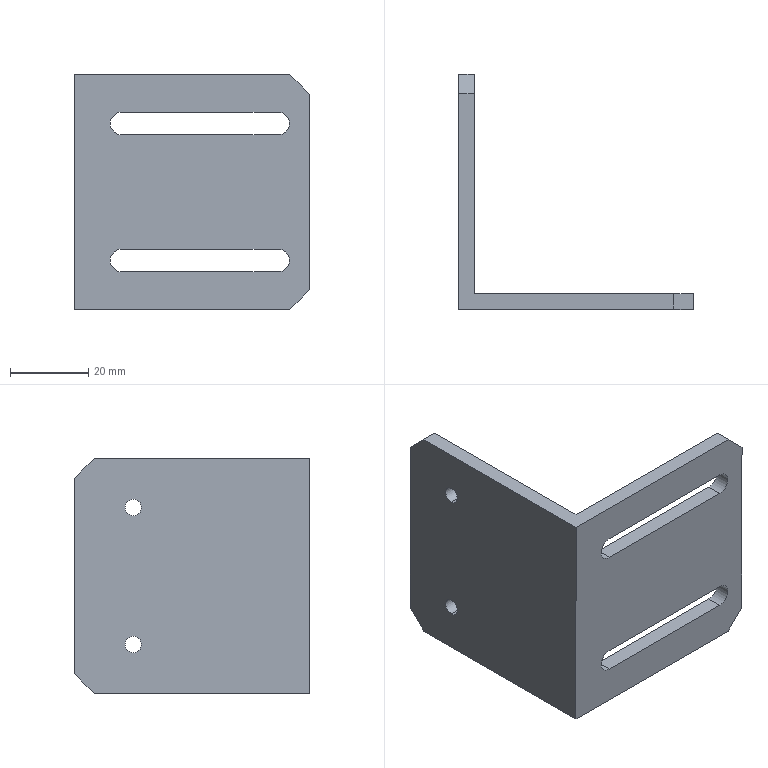Part | SolidWorks | features HoleWzd 2, Chamfer 1, Extrusion 1 | 1 solid | 24 faces | box 60 x 60 x 60 mm | volume 25462 mm3 | plane 16 | cylinder 8 | commonest cylinder face diameters 4.2 x4 5.8 x4
STEP:
#1=CARTESIAN_POINT('',(0.,45.,19.6));
#2=VERTEX_POINT('',#1);
#3=CARTESIAN_POINT('',(0.,45.,15.4));
#4=VERTEX_POINT('',#3);
#5=CARTESIAN_POINT('',(0.,45.,17.5));
#6=DIRECTION('',(1.,0.,0.));
#7=DIRECTION('',(0.,0.,-1.));
#8=AXIS2_PLACEMENT_3D('',#5,#6,#7);
#9=CIRCLE('',#8,2.1);
#10=EDGE_CURVE('',#2,#4,#9,.T.);
#11=ORIENTED_EDGE('',*,*,#10,.F.);
#12=CARTESIAN_POINT('',(4.,45.,19.6));
#13=VERTEX_POINT('',#12);
#14=CARTESIAN_POINT('',(4.,45.,19.6));
#15=DIRECTION('',(1.,0.,0.));
#16=VECTOR('',#15,1000.);
#17=LINE('',#14,#16);
#18=EDGE_CURVE('',#2,#13,#17,.T.);
#19=ORIENTED_EDGE('',*,*,#18,.T.);
#20=CARTESIAN_POINT('',(4.,45.,15.4));
#21=VERTEX_POINT('',#20);
#22=CARTESIAN_POINT('',(4.,45.,17.5));
#23=DIRECTION('',(1.,0.,0.));
#24=DIRECTION('',(0.,0.,-1.));
#25=AXIS2_PLACEMENT_3D('',#22,#23,#24);
#26=CIRCLE('',#25,2.1);
#27=EDGE_CURVE('',#13,#21,#26,.T.);
#28=ORIENTED_EDGE('',*,*,#27,.T.);
#29=CARTESIAN_POINT('',(4.,45.,15.4));
#30=DIRECTION('',(1.,0.,0.));
#31=VECTOR('',#30,1000.);
#32=LINE('',#29,#31);
#33=EDGE_CURVE('',#4,#21,#32,.T.);
#34=ORIENTED_EDGE('',*,*,#33,.F.);
#35=EDGE_LOOP('',(#11,#19,#28,#34));
#36=FACE_OUTER_BOUND('',#35,.T.);
#37=CARTESIAN_POINT('',(4.,45.,17.5));
#38=DIRECTION('',(1.,0.,0.));
#39=DIRECTION('',(0.,0.,-1.));
#40=AXIS2_PLACEMENT_3D('',#37,#38,#39);
#41=CYLINDRICAL_SURFACE('',#40,2.1);
#42=ADVANCED_FACE('',(#36),#41,.F.);
#43=CARTESIAN_POINT('',(0.,45.,-15.4));
#44=VERTEX_POINT('',#43);
#45=CARTESIAN_POINT('',(0.,45.,-19.6));
#46=VERTEX_POINT('',#45);
#47=CARTESIAN_POINT('',(0.,45.,-17.5));
#48=DIRECTION('',(1.,0.,0.));
#49=DIRECTION('',(0.,0.,-1.));
#50=AXIS2_PLACEMENT_3D('',#47,#48,#49);
#51=CIRCLE('',#50,2.1);
#52=EDGE_CURVE('',#44,#46,#51,.T.);
#53=ORIENTED_EDGE('',*,*,#52,.F.);
#54=CARTESIAN_POINT('',(4.,45.,-15.4));
#55=VERTEX_POINT('',#54);
#56=CARTESIAN_POINT('',(4.,45.,-15.4));
#57=DIRECTION('',(1.,0.,0.));
#58=VECTOR('',#57,1000.);
#59=LINE('',#56,#58);
#60=EDGE_CURVE('',#44,#55,#59,.T.);
#61=ORIENTED_EDGE('',*,*,#60,.T.);
#62=CARTESIAN_POINT('',(4.,45.,-19.6));
#63=VERTEX_POINT('',#62);
#64=CARTESIAN_POINT('',(4.,45.,-17.5));
#65=DIRECTION('',(1.,0.,0.));
#66=DIRECTION('',(0.,0.,-1.));
#67=AXIS2_PLACEMENT_3D('',#64,#65,#66);
#68=CIRCLE('',#67,2.1);
#69=EDGE_CURVE('',#55,#63,#68,.T.);
#70=ORIENTED_EDGE('',*,*,#69,.T.);
#71=CARTESIAN_POINT('',(4.,45.,-19.6));
#72=DIRECTION('',(1.,0.,0.));
#73=VECTOR('',#72,1000.);
#74=LINE('',#71,#73);
#75=EDGE_CURVE('',#46,#63,#74,.T.);
#76=ORIENTED_EDGE('',*,*,#75,.F.);
#77=EDGE_LOOP('',(#53,#61,#70,#76));
#78=FACE_OUTER_BOUND('',#77,.T.);
#79=CARTESIAN_POINT('',(4.,45.,-17.5));
#80=DIRECTION('',(1.,0.,0.));
#81=DIRECTION('',(0.,0.,-1.));
#82=AXIS2_PLACEMENT_3D('',#79,#80,#81);
#83=CYLINDRICAL_SURFACE('',#82,2.1);
#84=ADVANCED_FACE('',(#78),#83,.F.);
#85=CARTESIAN_POINT('',(12.,0.,-20.4));
#86=VERTEX_POINT('',#85);
#87=CARTESIAN_POINT('',(52.,0.,-20.4));
#88=VERTEX_POINT('',#87);
#89=CARTESIAN_POINT('',(12.,0.,-20.4));
#90=DIRECTION('',(1.,0.,0.));
#91=VECTOR('',#90,1000.);
#92=LINE('',#89,#91);
#93=EDGE_CURVE('',#86,#88,#92,.T.);
#94=ORIENTED_EDGE('',*,*,#93,.F.);
#95=CARTESIAN_POINT('',(12.,0.,-14.6));
#96=VERTEX_POINT('',#95);
#97=CARTESIAN_POINT('',(12.,0.,-17.5));
#98=DIRECTION('',(0.,1.,0.));
#99=DIRECTION('',(0.,0.,1.));
#100=AXIS2_PLACEMENT_3D('',#97,#98,#99);
#101=CIRCLE('',#100,2.9);
#102=EDGE_CURVE('',#86,#96,#101,.T.);
#103=ORIENTED_EDGE('',*,*,#102,.T.);
#104=CARTESIAN_POINT('',(52.,0.,-14.6));
#105=VERTEX_POINT('',#104);
#106=CARTESIAN_POINT('',(12.,0.,-14.6));
#107=DIRECTION('',(1.,0.,0.));
#108=VECTOR('',#107,1000.);
#109=LINE('',#106,#108);
#110=EDGE_CURVE('',#96,#105,#109,.T.);
#111=ORIENTED_EDGE('',*,*,#110,.T.);
#112=CARTESIAN_POINT('',(52.,0.,-17.5));
#113=DIRECTION('',(0.,1.,0.));
#114=DIRECTION('',(0.,0.,1.));
#115=AXIS2_PLACEMENT_3D('',#112,#113,#114);
#116=CIRCLE('',#115,2.9);
#117=EDGE_CURVE('',#105,#88,#116,.T.);
#118=ORIENTED_EDGE('',*,*,#117,.T.);
#119=EDGE_LOOP('',(#94,#103,#111,#118));
#120=FACE_BOUND('',#119,.T.);
#121=CARTESIAN_POINT('',(12.,0.,14.6));
#122=VERTEX_POINT('',#121);
#123=CARTESIAN_POINT('',(12.,0.,20.4));
#124=VERTEX_POINT('',#123);
#125=CARTESIAN_POINT('',(12.,0.,17.5));
#126=DIRECTION('',(0.,1.,0.));
#127=DIRECTION('',(0.,0.,1.));
#128=AXIS2_PLACEMENT_3D('',#125,#126,#127);
#129=CIRCLE('',#128,2.9);
#130=EDGE_CURVE('',#122,#124,#129,.T.);
#131=ORIENTED_EDGE('',*,*,#130,.T.);
#132=CARTESIAN_POINT('',(52.,0.,20.4));
#133=VERTEX_POINT('',#132);
#134=CARTESIAN_POINT('',(12.,0.,20.4));
#135=DIRECTION('',(1.,0.,0.));
#136=VECTOR('',#135,1000.);
#137=LINE('',#134,#136);
#138=EDGE_CURVE('',#124,#133,#137,.T.);
#139=ORIENTED_EDGE('',*,*,#138,.T.);
#140=CARTESIAN_POINT('',(52.,0.,14.6));
#141=VERTEX_POINT('',#140);
#142=CARTESIAN_POINT('',(52.,0.,17.5));
#143=DIRECTION('',(0.,1.,0.));
#144=DIRECTION('',(0.,0.,1.));
#145=AXIS2_PLACEMENT_3D('',#142,#143,#144);
#146=CIRCLE('',#145,2.9);
#147=EDGE_CURVE('',#133,#141,#146,.T.);
#148=ORIENTED_EDGE('',*,*,#147,.T.);
#149=CARTESIAN_POINT('',(12.,0.,14.6));
#150=DIRECTION('',(1.,0.,0.));
#151=VECTOR('',#150,1000.);
#152=LINE('',#149,#151);
#153=EDGE_CURVE('',#122,#141,#152,.T.);
#154=ORIENTED_EDGE('',*,*,#153,.F.);
#155=EDGE_LOOP('',(#131,#139,#148,#154));
#156=FACE_BOUND('',#155,.T.);
#157=CARTESIAN_POINT('',(60.,0.,25.));
#158=VERTEX_POINT('',#157);
#159=CARTESIAN_POINT('',(60.,0.,-25.));
#160=VERTEX_POINT('',#159);
#161=CARTESIAN_POINT('',(60.,0.,30.));
#162=DIRECTION('',(0.,0.,-1.));
#163=VECTOR('',#162,1000.);
#164=LINE('',#161,#163);
#165=EDGE_CURVE('',#158,#160,#164,.T.);
#166=ORIENTED_EDGE('',*,*,#165,.F.);
#167=CARTESIAN_POINT('',(55.,0.,30.));
#168=VERTEX_POINT('',#167);
#169=CARTESIAN_POINT('',(55.,0.,30.));
#170=DIRECTION('',(-0.7071,0.,0.7071));
#171=VECTOR('',#170,1000.);
#172=LINE('',#169,#171);
#173=EDGE_CURVE('',#158,#168,#172,.T.);
#174=ORIENTED_EDGE('',*,*,#173,.T.);
#175=CARTESIAN_POINT('',(0.,0.,30.));
#176=VERTEX_POINT('',#175);
#177=CARTESIAN_POINT('',(60.,0.,30.));
#178=DIRECTION('',(1.,0.,0.));
#179=VECTOR('',#178,1000.);
#180=LINE('',#177,#179);
#181=EDGE_CURVE('',#176,#168,#180,.T.);
#182=ORIENTED_EDGE('',*,*,#181,.F.);
#183=CARTESIAN_POINT('',(0.,0.,-30.));
#184=VERTEX_POINT('',#183);
#185=CARTESIAN_POINT('',(0.,0.,30.));
#186=DIRECTION('',(0.,0.,-1.));
#187=VECTOR('',#186,1000.);
#188=LINE('',#185,#187);
#189=EDGE_CURVE('',#176,#184,#188,.T.);
#190=ORIENTED_EDGE('',*,*,#189,.T.);
#191=CARTESIAN_POINT('',(55.,0.,-30.));
#192=VERTEX_POINT('',#191);
#193=CARTESIAN_POINT('',(60.,0.,-30.));
#194=DIRECTION('',(1.,0.,0.));
#195=VECTOR('',#194,1000.);
#196=LINE('',#193,#195);
#197=EDGE_CURVE('',#184,#192,#196,.T.);
#198=ORIENTED_EDGE('',*,*,#197,.T.);
#199=CARTESIAN_POINT('',(60.,0.,-25.));
#200=DIRECTION('',(0.7071,0.,0.7071));
#201=VECTOR('',#200,1000.);
#202=LINE('',#199,#201);
#203=EDGE_CURVE('',#192,#160,#202,.T.);
#204=ORIENTED_EDGE('',*,*,#203,.T.);
#205=EDGE_LOOP('',(#166,#174,#182,#190,#198,#204));
#206=FACE_OUTER_BOUND('',#205,.T.);
#207=CARTESIAN_POINT('',(60.,0.,30.));
#208=DIRECTION('',(0.,1.,0.));
#209=DIRECTION('',(-1.,0.,0.));
#210=AXIS2_PLACEMENT_3D('',#207,#208,#209);
#211=PLANE('',#210);
#212=ADVANCED_FACE('',(#120,#156,#206),#211,.F.);
#213=CARTESIAN_POINT('',(60.,4.,25.));
#214=VERTEX_POINT('',#213);
#215=CARTESIAN_POINT('',(60.,4.,-25.));
#216=VERTEX_POINT('',#215);
#217=CARTESIAN_POINT('',(60.,4.,30.));
#218=DIRECTION('',(0.,0.,-1.));
#219=VECTOR('',#218,1000.);
#220=LINE('',#217,#219);
#221=EDGE_CURVE('',#214,#216,#220,.T.);
#222=ORIENTED_EDGE('',*,*,#221,.F.);
#223=CARTESIAN_POINT('',(60.,4.,25.));
#224=DIRECTION('',(0.,-1.,0.));
#225=VECTOR('',#224,1000.);
#226=LINE('',#223,#225);
#227=EDGE_CURVE('',#214,#158,#226,.T.);
#228=ORIENTED_EDGE('',*,*,#227,.T.);
#229=ORIENTED_EDGE('',*,*,#165,.T.);
#230=CARTESIAN_POINT('',(60.,4.,-25.));
#231=DIRECTION('',(0.,1.,0.));
#232=VECTOR('',#231,1000.);
#233=LINE('',#230,#232);
#234=EDGE_CURVE('',#160,#216,#233,.T.);
#235=ORIENTED_EDGE('',*,*,#234,.T.);
#236=EDGE_LOOP('',(#222,#228,#229,#235));
#237=FACE_OUTER_BOUND('',#236,.T.);
#238=CARTESIAN_POINT('',(60.,4.,30.));
#239=DIRECTION('',(-1.,0.,0.));
#240=DIRECTION('',(0.,0.,1.));
#241=AXIS2_PLACEMENT_3D('',#238,#239,#240);
#242=PLANE('',#241);
#243=ADVANCED_FACE('',(#237),#242,.F.);
#244=CARTESIAN_POINT('',(12.,4.,-20.4));
#245=VERTEX_POINT('',#244);
#246=CARTESIAN_POINT('',(12.,4.,-14.6));
#247=VERTEX_POINT('',#246);
#248=CARTESIAN_POINT('',(12.,4.,-17.5));
#249=DIRECTION('',(0.,1.,0.));
#250=DIRECTION('',(0.,0.,1.));
#251=AXIS2_PLACEMENT_3D('',#248,#249,#250);
#252=CIRCLE('',#251,2.9);
#253=EDGE_CURVE('',#245,#247,#252,.T.);
#254=ORIENTED_EDGE('',*,*,#253,.F.);
#255=CARTESIAN_POINT('',(52.,4.,-20.4));
#256=VERTEX_POINT('',#255);
#257=CARTESIAN_POINT('',(12.,4.,-20.4));
#258=DIRECTION('',(1.,0.,0.));
#259=VECTOR('',#258,1000.);
#260=LINE('',#257,#259);
#261=EDGE_CURVE('',#245,#256,#260,.T.);
#262=ORIENTED_EDGE('',*,*,#261,.T.);
#263=CARTESIAN_POINT('',(52.,4.,-14.6));
#264=VERTEX_POINT('',#263);
#265=CARTESIAN_POINT('',(52.,4.,-17.5));
#266=DIRECTION('',(0.,1.,0.));
#267=DIRECTION('',(0.,0.,1.));
#268=AXIS2_PLACEMENT_3D('',#265,#266,#267);
#269=CIRCLE('',#268,2.9);
#270=EDGE_CURVE('',#264,#256,#269,.T.);
#271=ORIENTED_EDGE('',*,*,#270,.F.);
#272=CARTESIAN_POINT('',(12.,4.,-14.6));
#273=DIRECTION('',(1.,0.,0.));
#274=VECTOR('',#273,1000.);
#275=LINE('',#272,#274);
#276=EDGE_CURVE('',#247,#264,#275,.T.);
#277=ORIENTED_EDGE('',*,*,#276,.F.);
#278=EDGE_LOOP('',(#254,#262,#271,#277));
#279=FACE_BOUND('',#278,.T.);
#280=CARTESIAN_POINT('',(12.,4.,14.6));
#281=VERTEX_POINT('',#280);
#282=CARTESIAN_POINT('',(52.,4.,14.6));
#283=VERTEX_POINT('',#282);
#284=CARTESIAN_POINT('',(12.,4.,14.6));
#285=DIRECTION('',(1.,0.,0.));
#286=VECTOR('',#285,1000.);
#287=LINE('',#284,#286);
#288=EDGE_CURVE('',#281,#283,#287,.T.);
#289=ORIENTED_EDGE('',*,*,#288,.T.);
#290=CARTESIAN_POINT('',(52.,4.,20.4));
#291=VERTEX_POINT('',#290);
#292=CARTESIAN_POINT('',(52.,4.,17.5));
#293=DIRECTION('',(0.,1.,0.));
#294=DIRECTION('',(0.,0.,1.));
#295=AXIS2_PLACEMENT_3D('',#292,#293,#294);
#296=CIRCLE('',#295,2.9);
#297=EDGE_CURVE('',#291,#283,#296,.T.);
#298=ORIENTED_EDGE('',*,*,#297,.F.);
#299=CARTESIAN_POINT('',(12.,4.,20.4));
#300=VERTEX_POINT('',#299);
#301=CARTESIAN_POINT('',(12.,4.,20.4));
#302=DIRECTION('',(1.,0.,0.));
#303=VECTOR('',#302,1000.);
#304=LINE('',#301,#303);
#305=EDGE_CURVE('',#300,#291,#304,.T.);
#306=ORIENTED_EDGE('',*,*,#305,.F.);
#307=CARTESIAN_POINT('',(12.,4.,17.5));
#308=DIRECTION('',(0.,1.,0.));
#309=DIRECTION('',(0.,0.,1.));
#310=AXIS2_PLACEMENT_3D('',#307,#308,#309);
#311=CIRCLE('',#310,2.9);
#312=EDGE_CURVE('',#281,#300,#311,.T.);
#313=ORIENTED_EDGE('',*,*,#312,.F.);
#314=EDGE_LOOP('',(#289,#298,#306,#313));
#315=FACE_BOUND('',#314,.T.);
#316=CARTESIAN_POINT('',(55.,4.,30.));
#317=VERTEX_POINT('',#316);
#318=CARTESIAN_POINT('',(4.,4.,30.));
#319=VERTEX_POINT('',#318);
#320=CARTESIAN_POINT('',(4.,4.,30.));
#321=DIRECTION('',(-1.,0.,0.));
#322=VECTOR('',#321,1000.);
#323=LINE('',#320,#322);
#324=EDGE_CURVE('',#317,#319,#323,.T.);
#325=ORIENTED_EDGE('',*,*,#324,.F.);
#326=CARTESIAN_POINT('',(55.,4.,30.));
#327=DIRECTION('',(0.7071,0.,-0.7071));
#328=VECTOR('',#327,1000.);
#329=LINE('',#326,#328);
#330=EDGE_CURVE('',#317,#214,#329,.T.);
#331=ORIENTED_EDGE('',*,*,#330,.T.);
#332=ORIENTED_EDGE('',*,*,#221,.T.);
#333=CARTESIAN_POINT('',(55.,4.,-30.));
#334=VERTEX_POINT('',#333);
#335=CARTESIAN_POINT('',(60.,4.,-25.));
#336=DIRECTION('',(-0.7071,0.,-0.7071));
#337=VECTOR('',#336,1000.);
#338=LINE('',#335,#337);
#339=EDGE_CURVE('',#216,#334,#338,.T.);
#340=ORIENTED_EDGE('',*,*,#339,.T.);
#341=CARTESIAN_POINT('',(4.,4.,-30.));
#342=VERTEX_POINT('',#341);
#343=CARTESIAN_POINT('',(4.,4.,-30.));
#344=DIRECTION('',(-1.,0.,0.));
#345=VECTOR('',#344,1000.);
#346=LINE('',#343,#345);
#347=EDGE_CURVE('',#334,#342,#346,.T.);
#348=ORIENTED_EDGE('',*,*,#347,.T.);
#349=CARTESIAN_POINT('',(4.,4.,30.));
#350=DIRECTION('',(0.,0.,-1.));
#351=VECTOR('',#350,1000.);
#352=LINE('',#349,#351);
#353=EDGE_CURVE('',#319,#342,#352,.T.);
#354=ORIENTED_EDGE('',*,*,#353,.F.);
#355=EDGE_LOOP('',(#325,#331,#332,#340,#348,#354));
#356=FACE_OUTER_BOUND('',#355,.T.);
#357=CARTESIAN_POINT('',(4.,4.,30.));
#358=DIRECTION('',(0.,-1.,0.));
#359=DIRECTION('',(0.,0.,-1.));
#360=AXIS2_PLACEMENT_3D('',#357,#358,#359);
#361=PLANE('',#360);
#362=ADVANCED_FACE('',(#279,#315,#356),#361,.F.);
#363=CARTESIAN_POINT('',(4.,45.,17.5));
#364=DIRECTION('',(1.,0.,0.));
#365=DIRECTION('',(0.,0.,-1.));
#366=AXIS2_PLACEMENT_3D('',#363,#364,#365);
#367=CIRCLE('',#366,2.1);
#368=EDGE_CURVE('',#21,#13,#367,.T.);
#369=ORIENTED_EDGE('',*,*,#368,.F.);
#370=ORIENTED_EDGE('',*,*,#27,.F.);
#371=EDGE_LOOP('',(#369,#370));
#372=FACE_BOUND('',#371,.T.);
#373=CARTESIAN_POINT('',(4.,45.,-17.5));
#374=DIRECTION('',(1.,0.,0.));
#375=DIRECTION('',(0.,0.,-1.));
#376=AXIS2_PLACEMENT_3D('',#373,#374,#375);
#377=CIRCLE('',#376,2.1);
#378=EDGE_CURVE('',#63,#55,#377,.T.);
#379=ORIENTED_EDGE('',*,*,#378,.F.);
#380=ORIENTED_EDGE('',*,*,#69,.F.);
#381=EDGE_LOOP('',(#379,#380));
#382=FACE_BOUND('',#381,.T.);
#383=CARTESIAN_POINT('',(4.,55.,-30.));
#384=VERTEX_POINT('',#383);
#385=CARTESIAN_POINT('',(4.,60.,-30.));
#386=DIRECTION('',(0.,1.,0.));
#387=VECTOR('',#386,1000.);
#388=LINE('',#385,#387);
#389=EDGE_CURVE('',#342,#384,#388,.T.);
#390=ORIENTED_EDGE('',*,*,#389,.T.);
#391=CARTESIAN_POINT('',(4.,60.,-25.));
#392=VERTEX_POINT('',#391);
#393=CARTESIAN_POINT('',(4.,60.,-25.));
#394=DIRECTION('',(0.,0.7071,0.7071));
#395=VECTOR('',#394,1000.);
#396=LINE('',#393,#395);
#397=EDGE_CURVE('',#384,#392,#396,.T.);
#398=ORIENTED_EDGE('',*,*,#397,.T.);
#399=CARTESIAN_POINT('',(4.,60.,25.));
#400=VERTEX_POINT('',#399);
#401=CARTESIAN_POINT('',(4.,60.,30.));
#402=DIRECTION('',(0.,0.,-1.));
#403=VECTOR('',#402,1000.);
#404=LINE('',#401,#403);
#405=EDGE_CURVE('',#400,#392,#404,.T.);
#406=ORIENTED_EDGE('',*,*,#405,.F.);
#407=CARTESIAN_POINT('',(4.,55.,30.));
#408=VERTEX_POINT('',#407);
#409=CARTESIAN_POINT('',(4.,55.,30.));
#410=DIRECTION('',(0.,-0.7071,0.7071));
#411=VECTOR('',#410,1000.);
#412=LINE('',#409,#411);
#413=EDGE_CURVE('',#400,#408,#412,.T.);
#414=ORIENTED_EDGE('',*,*,#413,.T.);
#415=CARTESIAN_POINT('',(4.,60.,30.));
#416=DIRECTION('',(0.,1.,0.));
#417=VECTOR('',#416,1000.);
#418=LINE('',#415,#417);
#419=EDGE_CURVE('',#319,#408,#418,.T.);
#420=ORIENTED_EDGE('',*,*,#419,.F.);
#421=ORIENTED_EDGE('',*,*,#353,.T.);
#422=EDGE_LOOP('',(#390,#398,#406,#414,#420,#421));
#423=FACE_OUTER_BOUND('',#422,.T.);
#424=CARTESIAN_POINT('',(4.,60.,30.));
#425=DIRECTION('',(-1.,0.,0.));
#426=DIRECTION('',(0.,-1.,0.));
#427=AXIS2_PLACEMENT_3D('',#424,#425,#426);
#428=PLANE('',#427);
#429=ADVANCED_FACE('',(#372,#382,#423),#428,.F.);
#430=ORIENTED_EDGE('',*,*,#405,.T.);
#431=CARTESIAN_POINT('',(0.,60.,-25.));
#432=VERTEX_POINT('',#431);
#433=CARTESIAN_POINT('',(0.,60.,-25.));
#434=DIRECTION('',(-1.,0.,0.));
#435=VECTOR('',#434,1000.);
#436=LINE('',#433,#435);
#437=EDGE_CURVE('',#392,#432,#436,.T.);
#438=ORIENTED_EDGE('',*,*,#437,.T.);
#439=CARTESIAN_POINT('',(0.,60.,25.));
#440=VERTEX_POINT('',#439);
#441=CARTESIAN_POINT('',(0.,60.,30.));
#442=DIRECTION('',(0.,0.,-1.));
#443=VECTOR('',#442,1000.);
#444=LINE('',#441,#443);
#445=EDGE_CURVE('',#440,#432,#444,.T.);
#446=ORIENTED_EDGE('',*,*,#445,.F.);
#447=CARTESIAN_POINT('',(0.,60.,25.));
#448=DIRECTION('',(1.,0.,0.));
#449=VECTOR('',#448,1000.);
#450=LINE('',#447,#449);
#451=EDGE_CURVE('',#440,#400,#450,.T.);
#452=ORIENTED_EDGE('',*,*,#451,.T.);
#453=EDGE_LOOP('',(#430,#438,#446,#452));
#454=FACE_OUTER_BOUND('',#453,.T.);
#455=CARTESIAN_POINT('',(0.,60.,30.));
#456=DIRECTION('',(0.,-1.,0.));
#457=DIRECTION('',(0.,0.,-1.));
#458=AXIS2_PLACEMENT_3D('',#455,#456,#457);
#459=PLANE('',#458);
#460=ADVANCED_FACE('',(#454),#459,.F.);
#461=CARTESIAN_POINT('',(0.,45.,17.5));
#462=DIRECTION('',(1.,0.,0.));
#463=DIRECTION('',(0.,0.,-1.));
#464=AXIS2_PLACEMENT_3D('',#461,#462,#463);
#465=CIRCLE('',#464,2.1);
#466=EDGE_CURVE('',#4,#2,#465,.T.);
#467=ORIENTED_EDGE('',*,*,#466,.T.);
#468=ORIENTED_EDGE('',*,*,#10,.T.);
#469=EDGE_LOOP('',(#467,#468));
#470=FACE_BOUND('',#469,.T.);
#471=CARTESIAN_POINT('',(0.,45.,-17.5));
#472=DIRECTION('',(1.,0.,0.));
#473=DIRECTION('',(0.,0.,-1.));
#474=AXIS2_PLACEMENT_3D('',#471,#472,#473);
#475=CIRCLE('',#474,2.1);
#476=EDGE_CURVE('',#46,#44,#475,.T.);
#477=ORIENTED_EDGE('',*,*,#476,.T.);
#478=ORIENTED_EDGE('',*,*,#52,.T.);
#479=EDGE_LOOP('',(#477,#478));
#480=FACE_BOUND('',#479,.T.);
#481=ORIENTED_EDGE('',*,*,#445,.T.);
#482=CARTESIAN_POINT('',(0.,55.,-30.));
#483=VERTEX_POINT('',#482);
#484=CARTESIAN_POINT('',(0.,60.,-25.));
#485=DIRECTION('',(0.,-0.7071,-0.7071));
#486=VECTOR('',#485,1000.);
#487=LINE('',#484,#486);
#488=EDGE_CURVE('',#432,#483,#487,.T.);
#489=ORIENTED_EDGE('',*,*,#488,.T.);
#490=CARTESIAN_POINT('',(0.,0.,-30.));
#491=DIRECTION('',(0.,-1.,0.));
#492=VECTOR('',#491,1000.);
#493=LINE('',#490,#492);
#494=EDGE_CURVE('',#483,#184,#493,.T.);
#495=ORIENTED_EDGE('',*,*,#494,.T.);
#496=ORIENTED_EDGE('',*,*,#189,.F.);
#497=CARTESIAN_POINT('',(0.,55.,30.));
#498=VERTEX_POINT('',#497);
#499=CARTESIAN_POINT('',(0.,0.,30.));
#500=DIRECTION('',(0.,-1.,0.));
#501=VECTOR('',#500,1000.);
#502=LINE('',#499,#501);
#503=EDGE_CURVE('',#498,#176,#502,.T.);
#504=ORIENTED_EDGE('',*,*,#503,.F.);
#505=CARTESIAN_POINT('',(0.,55.,30.));
#506=DIRECTION('',(0.,0.7071,-0.7071));
#507=VECTOR('',#506,1000.);
#508=LINE('',#505,#507);
#509=EDGE_CURVE('',#498,#440,#508,.T.);
#510=ORIENTED_EDGE('',*,*,#509,.T.);
#511=EDGE_LOOP('',(#481,#489,#495,#496,#504,#510));
#512=FACE_OUTER_BOUND('',#511,.T.);
#513=CARTESIAN_POINT('',(0.,0.,30.));
#514=DIRECTION('',(1.,0.,0.));
#515=DIRECTION('',(0.,0.,-1.));
#516=AXIS2_PLACEMENT_3D('',#513,#514,#515);
#517=PLANE('',#516);
#518=ADVANCED_FACE('',(#470,#480,#512),#517,.F.);
#519=ORIENTED_EDGE('',*,*,#181,.T.);
#520=CARTESIAN_POINT('',(55.,0.,30.));
#521=DIRECTION('',(0.,1.,0.));
#522=VECTOR('',#521,1000.);
#523=LINE('',#520,#522);
#524=EDGE_CURVE('',#168,#317,#523,.T.);
#525=ORIENTED_EDGE('',*,*,#524,.T.);
#526=ORIENTED_EDGE('',*,*,#324,.T.);
#527=ORIENTED_EDGE('',*,*,#419,.T.);
#528=CARTESIAN_POINT('',(0.,55.,30.));
#529=DIRECTION('',(-1.,0.,0.));
#530=VECTOR('',#529,1000.);
#531=LINE('',#528,#530);
#532=EDGE_CURVE('',#408,#498,#531,.T.);
#533=ORIENTED_EDGE('',*,*,#532,.T.);
#534=ORIENTED_EDGE('',*,*,#503,.T.);
#535=EDGE_LOOP('',(#519,#525,#526,#527,#533,#534));
#536=FACE_OUTER_BOUND('',#535,.T.);
#537=CARTESIAN_POINT('',(0.,0.,30.));
#538=DIRECTION('',(0.,0.,-1.));
#539=DIRECTION('',(-1.,0.,0.));
#540=AXIS2_PLACEMENT_3D('',#537,#538,#539);
#541=PLANE('',#540);
#542=ADVANCED_FACE('',(#536),#541,.F.);
#543=ORIENTED_EDGE('',*,*,#347,.F.);
#544=CARTESIAN_POINT('',(55.,0.,-30.));
#545=DIRECTION('',(0.,-1.,0.));
#546=VECTOR('',#545,1000.);
#547=LINE('',#544,#546);
#548=EDGE_CURVE('',#334,#192,#547,.T.);
#549=ORIENTED_EDGE('',*,*,#548,.T.);
#550=ORIENTED_EDGE('',*,*,#197,.F.);
#551=ORIENTED_EDGE('',*,*,#494,.F.);
#552=CARTESIAN_POINT('',(4.,55.,-30.));
#553=DIRECTION('',(1.,0.,0.));
#554=VECTOR('',#553,1000.);
#555=LINE('',#552,#554);
#556=EDGE_CURVE('',#483,#384,#555,.T.);
#557=ORIENTED_EDGE('',*,*,#556,.T.);
#558=ORIENTED_EDGE('',*,*,#389,.F.);
#559=EDGE_LOOP('',(#543,#549,#550,#551,#557,#558));
#560=FACE_OUTER_BOUND('',#559,.T.);
#561=CARTESIAN_POINT('',(0.,0.,-30.));
#562=DIRECTION('',(0.,0.,-1.));
#563=DIRECTION('',(-1.,0.,0.));
#564=AXIS2_PLACEMENT_3D('',#561,#562,#563);
#565=PLANE('',#564);
#566=ADVANCED_FACE('',(#560),#565,.T.);
#567=ORIENTED_EDGE('',*,*,#60,.F.);
#568=ORIENTED_EDGE('',*,*,#476,.F.);
#569=ORIENTED_EDGE('',*,*,#75,.T.);
#570=ORIENTED_EDGE('',*,*,#378,.T.);
#571=EDGE_LOOP('',(#567,#568,#569,#570));
#572=FACE_OUTER_BOUND('',#571,.T.);
#573=CARTESIAN_POINT('',(4.,45.,-17.5));
#574=DIRECTION('',(1.,0.,0.));
#575=DIRECTION('',(0.,0.,-1.));
#576=AXIS2_PLACEMENT_3D('',#573,#574,#575);
#577=CYLINDRICAL_SURFACE('',#576,2.1);
#578=ADVANCED_FACE('',(#572),#577,.F.);
#579=ORIENTED_EDGE('',*,*,#18,.F.);
#580=ORIENTED_EDGE('',*,*,#466,.F.);
#581=ORIENTED_EDGE('',*,*,#33,.T.);
#582=ORIENTED_EDGE('',*,*,#368,.T.);
#583=EDGE_LOOP('',(#579,#580,#581,#582));
#584=FACE_OUTER_BOUND('',#583,.T.);
#585=CARTESIAN_POINT('',(4.,45.,17.5));
#586=DIRECTION('',(1.,0.,0.));
#587=DIRECTION('',(0.,0.,-1.));
#588=AXIS2_PLACEMENT_3D('',#585,#586,#587);
#589=CYLINDRICAL_SURFACE('',#588,2.1);
#590=ADVANCED_FACE('',(#584),#589,.F.);
#591=ORIENTED_EDGE('',*,*,#147,.F.);
#592=CARTESIAN_POINT('',(52.,4.,20.4));
#593=DIRECTION('',(0.,-1.,0.));
#594=VECTOR('',#593,1000.);
#595=LINE('',#592,#594);
#596=EDGE_CURVE('',#291,#133,#595,.T.);
#597=ORIENTED_EDGE('',*,*,#596,.F.);
#598=ORIENTED_EDGE('',*,*,#297,.T.);
#599=CARTESIAN_POINT('',(52.,4.,14.6));
#600=DIRECTION('',(0.,1.,0.));
#601=VECTOR('',#600,1000.);
#602=LINE('',#599,#601);
#603=EDGE_CURVE('',#141,#283,#602,.T.);
#604=ORIENTED_EDGE('',*,*,#603,.F.);
#605=EDGE_LOOP('',(#591,#597,#598,#604));
#606=FACE_OUTER_BOUND('',#605,.T.);
#607=CARTESIAN_POINT('',(52.,4.,17.5));
#608=DIRECTION('',(0.,1.,0.));
#609=DIRECTION('',(0.,0.,1.));
#610=AXIS2_PLACEMENT_3D('',#607,#608,#609);
#611=CYLINDRICAL_SURFACE('',#610,2.9);
#612=ADVANCED_FACE('',(#606),#611,.F.);
#613=ORIENTED_EDGE('',*,*,#312,.T.);
#614=CARTESIAN_POINT('',(12.,4.,20.4));
#615=DIRECTION('',(0.,1.,0.));
#616=VECTOR('',#615,1000.);
#617=LINE('',#614,#616);
#618=EDGE_CURVE('',#124,#300,#617,.T.);
#619=ORIENTED_EDGE('',*,*,#618,.F.);
#620=ORIENTED_EDGE('',*,*,#130,.F.);
#621=CARTESIAN_POINT('',(12.,4.,14.6));
#622=DIRECTION('',(0.,-1.,0.));
#623=VECTOR('',#622,1000.);
#624=LINE('',#621,#623);
#625=EDGE_CURVE('',#281,#122,#624,.T.);
#626=ORIENTED_EDGE('',*,*,#625,.F.);
#627=EDGE_LOOP('',(#613,#619,#620,#626));
#628=FACE_OUTER_BOUND('',#627,.T.);
#629=CARTESIAN_POINT('',(12.,4.,17.5));
#630=DIRECTION('',(0.,1.,0.));
#631=DIRECTION('',(0.,0.,1.));
#632=AXIS2_PLACEMENT_3D('',#629,#630,#631);
#633=CYLINDRICAL_SURFACE('',#632,2.9);
#634=ADVANCED_FACE('',(#628),#633,.F.);
#635=ORIENTED_EDGE('',*,*,#603,.T.);
#636=ORIENTED_EDGE('',*,*,#288,.F.);
#637=ORIENTED_EDGE('',*,*,#625,.T.);
#638=ORIENTED_EDGE('',*,*,#153,.T.);
#639=EDGE_LOOP('',(#635,#636,#637,#638));
#640=FACE_OUTER_BOUND('',#639,.T.);
#641=CARTESIAN_POINT('',(12.,4.,14.6));
#642=DIRECTION('',(0.,0.,-1.));
#643=DIRECTION('',(-1.,0.,0.));
#644=AXIS2_PLACEMENT_3D('',#641,#642,#643);
#645=PLANE('',#644);
#646=ADVANCED_FACE('',(#640),#645,.F.);
#647=ORIENTED_EDGE('',*,*,#596,.T.);
#648=ORIENTED_EDGE('',*,*,#138,.F.);
#649=ORIENTED_EDGE('',*,*,#618,.T.);
#650=ORIENTED_EDGE('',*,*,#305,.T.);
#651=EDGE_LOOP('',(#647,#648,#649,#650));
#652=FACE_OUTER_BOUND('',#651,.T.);
#653=CARTESIAN_POINT('',(12.,4.,20.4));
#654=DIRECTION('',(0.,0.,1.));
#655=DIRECTION('',(1.,0.,0.));
#656=AXIS2_PLACEMENT_3D('',#653,#654,#655);
#657=PLANE('',#656);
#658=ADVANCED_FACE('',(#652),#657,.F.);
#659=ORIENTED_EDGE('',*,*,#117,.F.);
#660=CARTESIAN_POINT('',(52.,4.,-14.6));
#661=DIRECTION('',(0.,-1.,0.));
#662=VECTOR('',#661,1000.);
#663=LINE('',#660,#662);
#664=EDGE_CURVE('',#264,#105,#663,.T.);
#665=ORIENTED_EDGE('',*,*,#664,.F.);
#666=ORIENTED_EDGE('',*,*,#270,.T.);
#667=CARTESIAN_POINT('',(52.,4.,-20.4));
#668=DIRECTION('',(0.,1.,0.));
#669=VECTOR('',#668,1000.);
#670=LINE('',#667,#669);
#671=EDGE_CURVE('',#88,#256,#670,.T.);
#672=ORIENTED_EDGE('',*,*,#671,.F.);
#673=EDGE_LOOP('',(#659,#665,#666,#672));
#674=FACE_OUTER_BOUND('',#673,.T.);
#675=CARTESIAN_POINT('',(52.,4.,-17.5));
#676=DIRECTION('',(0.,1.,0.));
#677=DIRECTION('',(0.,0.,1.));
#678=AXIS2_PLACEMENT_3D('',#675,#676,#677);
#679=CYLINDRICAL_SURFACE('',#678,2.9);
#680=ADVANCED_FACE('',(#674),#679,.F.);
#681=ORIENTED_EDGE('',*,*,#253,.T.);
#682=CARTESIAN_POINT('',(12.,4.,-14.6));
#683=DIRECTION('',(0.,1.,0.));
#684=VECTOR('',#683,1000.);
#685=LINE('',#682,#684);
#686=EDGE_CURVE('',#96,#247,#685,.T.);
#687=ORIENTED_EDGE('',*,*,#686,.F.);
#688=ORIENTED_EDGE('',*,*,#102,.F.);
#689=CARTESIAN_POINT('',(12.,4.,-20.4));
#690=DIRECTION('',(0.,-1.,0.));
#691=VECTOR('',#690,1000.);
#692=LINE('',#689,#691);
#693=EDGE_CURVE('',#245,#86,#692,.T.);
#694=ORIENTED_EDGE('',*,*,#693,.F.);
#695=EDGE_LOOP('',(#681,#687,#688,#694));
#696=FACE_OUTER_BOUND('',#695,.T.);
#697=CARTESIAN_POINT('',(12.,4.,-17.5));
#698=DIRECTION('',(0.,1.,0.));
#699=DIRECTION('',(0.,0.,1.));
#700=AXIS2_PLACEMENT_3D('',#697,#698,#699);
#701=CYLINDRICAL_SURFACE('',#700,2.9);
#702=ADVANCED_FACE('',(#696),#701,.F.);
#703=ORIENTED_EDGE('',*,*,#671,.T.);
#704=ORIENTED_EDGE('',*,*,#261,.F.);
#705=ORIENTED_EDGE('',*,*,#693,.T.);
#706=ORIENTED_EDGE('',*,*,#93,.T.);
#707=EDGE_LOOP('',(#703,#704,#705,#706));
#708=FACE_OUTER_BOUND('',#707,.T.);
#709=CARTESIAN_POINT('',(12.,4.,-20.4));
#710=DIRECTION('',(0.,0.,-1.));
#711=DIRECTION('',(-1.,0.,0.));
#712=AXIS2_PLACEMENT_3D('',#709,#710,#711);
#713=PLANE('',#712);
#714=ADVANCED_FACE('',(#708),#713,.F.);
#715=ORIENTED_EDGE('',*,*,#664,.T.);
#716=ORIENTED_EDGE('',*,*,#110,.F.);
#717=ORIENTED_EDGE('',*,*,#686,.T.);
#718=ORIENTED_EDGE('',*,*,#276,.T.);
#719=EDGE_LOOP('',(#715,#716,#717,#718));
#720=FACE_OUTER_BOUND('',#719,.T.);
#721=CARTESIAN_POINT('',(12.,4.,-14.6));
#722=DIRECTION('',(0.,0.,1.));
#723=DIRECTION('',(1.,0.,0.));
#724=AXIS2_PLACEMENT_3D('',#721,#722,#723);
#725=PLANE('',#724);
#726=ADVANCED_FACE('',(#720),#725,.F.);
#727=ORIENTED_EDGE('',*,*,#173,.F.);
#728=ORIENTED_EDGE('',*,*,#227,.F.);
#729=ORIENTED_EDGE('',*,*,#330,.F.);
#730=ORIENTED_EDGE('',*,*,#524,.F.);
#731=EDGE_LOOP('',(#727,#728,#729,#730));
#732=FACE_OUTER_BOUND('',#731,.T.);
#733=CARTESIAN_POINT('',(55.,0.,30.));
#734=DIRECTION('',(-0.7071,0.,-0.7071));
#735=DIRECTION('',(0.,1.,0.));
#736=AXIS2_PLACEMENT_3D('',#733,#734,#735);
#737=PLANE('',#736);
#738=ADVANCED_FACE('',(#732),#737,.F.);
#739=ORIENTED_EDGE('',*,*,#203,.F.);
#740=ORIENTED_EDGE('',*,*,#548,.F.);
#741=ORIENTED_EDGE('',*,*,#339,.F.);
#742=ORIENTED_EDGE('',*,*,#234,.F.);
#743=EDGE_LOOP('',(#739,#740,#741,#742));
#744=FACE_OUTER_BOUND('',#743,.T.);
#745=CARTESIAN_POINT('',(60.,4.,-25.));
#746=DIRECTION('',(0.7071,0.,-0.7071));
#747=DIRECTION('',(0.,-1.,0.));
#748=AXIS2_PLACEMENT_3D('',#745,#746,#747);
#749=PLANE('',#748);
#750=ADVANCED_FACE('',(#744),#749,.T.);
#751=ORIENTED_EDGE('',*,*,#397,.F.);
#752=ORIENTED_EDGE('',*,*,#556,.F.);
#753=ORIENTED_EDGE('',*,*,#488,.F.);
#754=ORIENTED_EDGE('',*,*,#437,.F.);
#755=EDGE_LOOP('',(#751,#752,#753,#754));
#756=FACE_OUTER_BOUND('',#755,.T.);
#757=CARTESIAN_POINT('',(0.,60.,-25.));
#758=DIRECTION('',(0.,0.7071,-0.7071));
#759=DIRECTION('',(1.,0.,0.));
#760=AXIS2_PLACEMENT_3D('',#757,#758,#759);
#761=PLANE('',#760);
#762=ADVANCED_FACE('',(#756),#761,.T.);
#763=ORIENTED_EDGE('',*,*,#413,.F.);
#764=ORIENTED_EDGE('',*,*,#451,.F.);
#765=ORIENTED_EDGE('',*,*,#509,.F.);
#766=ORIENTED_EDGE('',*,*,#532,.F.);
#767=EDGE_LOOP('',(#763,#764,#765,#766));
#768=FACE_OUTER_BOUND('',#767,.T.);
#769=CARTESIAN_POINT('',(0.,55.,30.));
#770=DIRECTION('',(0.,-0.7071,-0.7071));
#771=DIRECTION('',(-1.,0.,0.));
#772=AXIS2_PLACEMENT_3D('',#769,#770,#771);
#773=PLANE('',#772);
#774=ADVANCED_FACE('',(#768),#773,.F.);
#775=CLOSED_SHELL('',(#42,#84,#212,#243,#362,#429,#460,#518,#542,#566,#578,#590,#612,#634,#646,#658,#680,#702,#714,#726,#738,#750,#762,#774));
#776=MANIFOLD_SOLID_BREP('',#775);
#777=CARTESIAN_POINT('',(0.,0.,0.));
#778=DIRECTION('',(0.,0.,1.));
#779=DIRECTION('',(1.,0.,0.));
#780=AXIS2_PLACEMENT_3D('',#777,#778,#779);
#781=(LENGTH_UNIT()NAMED_UNIT(*)SI_UNIT(.MILLI.,.METRE.));
#782=UNCERTAINTY_MEASURE_WITH_UNIT(LENGTH_MEASURE(0.00001),#781,'','');
#783=(NAMED_UNIT(*)PLANE_ANGLE_UNIT()SI_UNIT($,.RADIAN.));
#784=(NAMED_UNIT(*)SI_UNIT($,.STERADIAN.)SOLID_ANGLE_UNIT());
#785=(GEOMETRIC_REPRESENTATION_CONTEXT(3)GLOBAL_UNCERTAINTY_ASSIGNED_CONTEXT((#782))GLOBAL_UNIT_ASSIGNED_CONTEXT((#781,#783,#784))REPRESENTATION_CONTEXT('',''));
#786=ADVANCED_BREP_SHAPE_REPRESENTATION('',(#776,#780),#785);